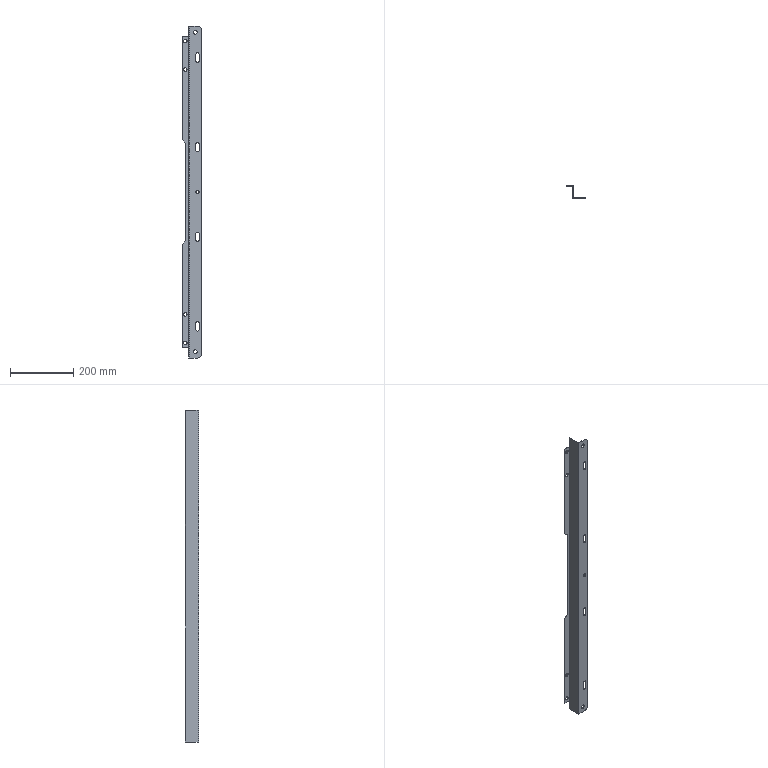Part | 1 solid | 70 faces | box 60 x 42 x 1050 mm | volume 146958 mm3 | plane 38 | cylinder 32 | commonest cylinder face diameters 10 x14 11 x8 12.5 x4 0.4 x2 3.4 x2 26 x2